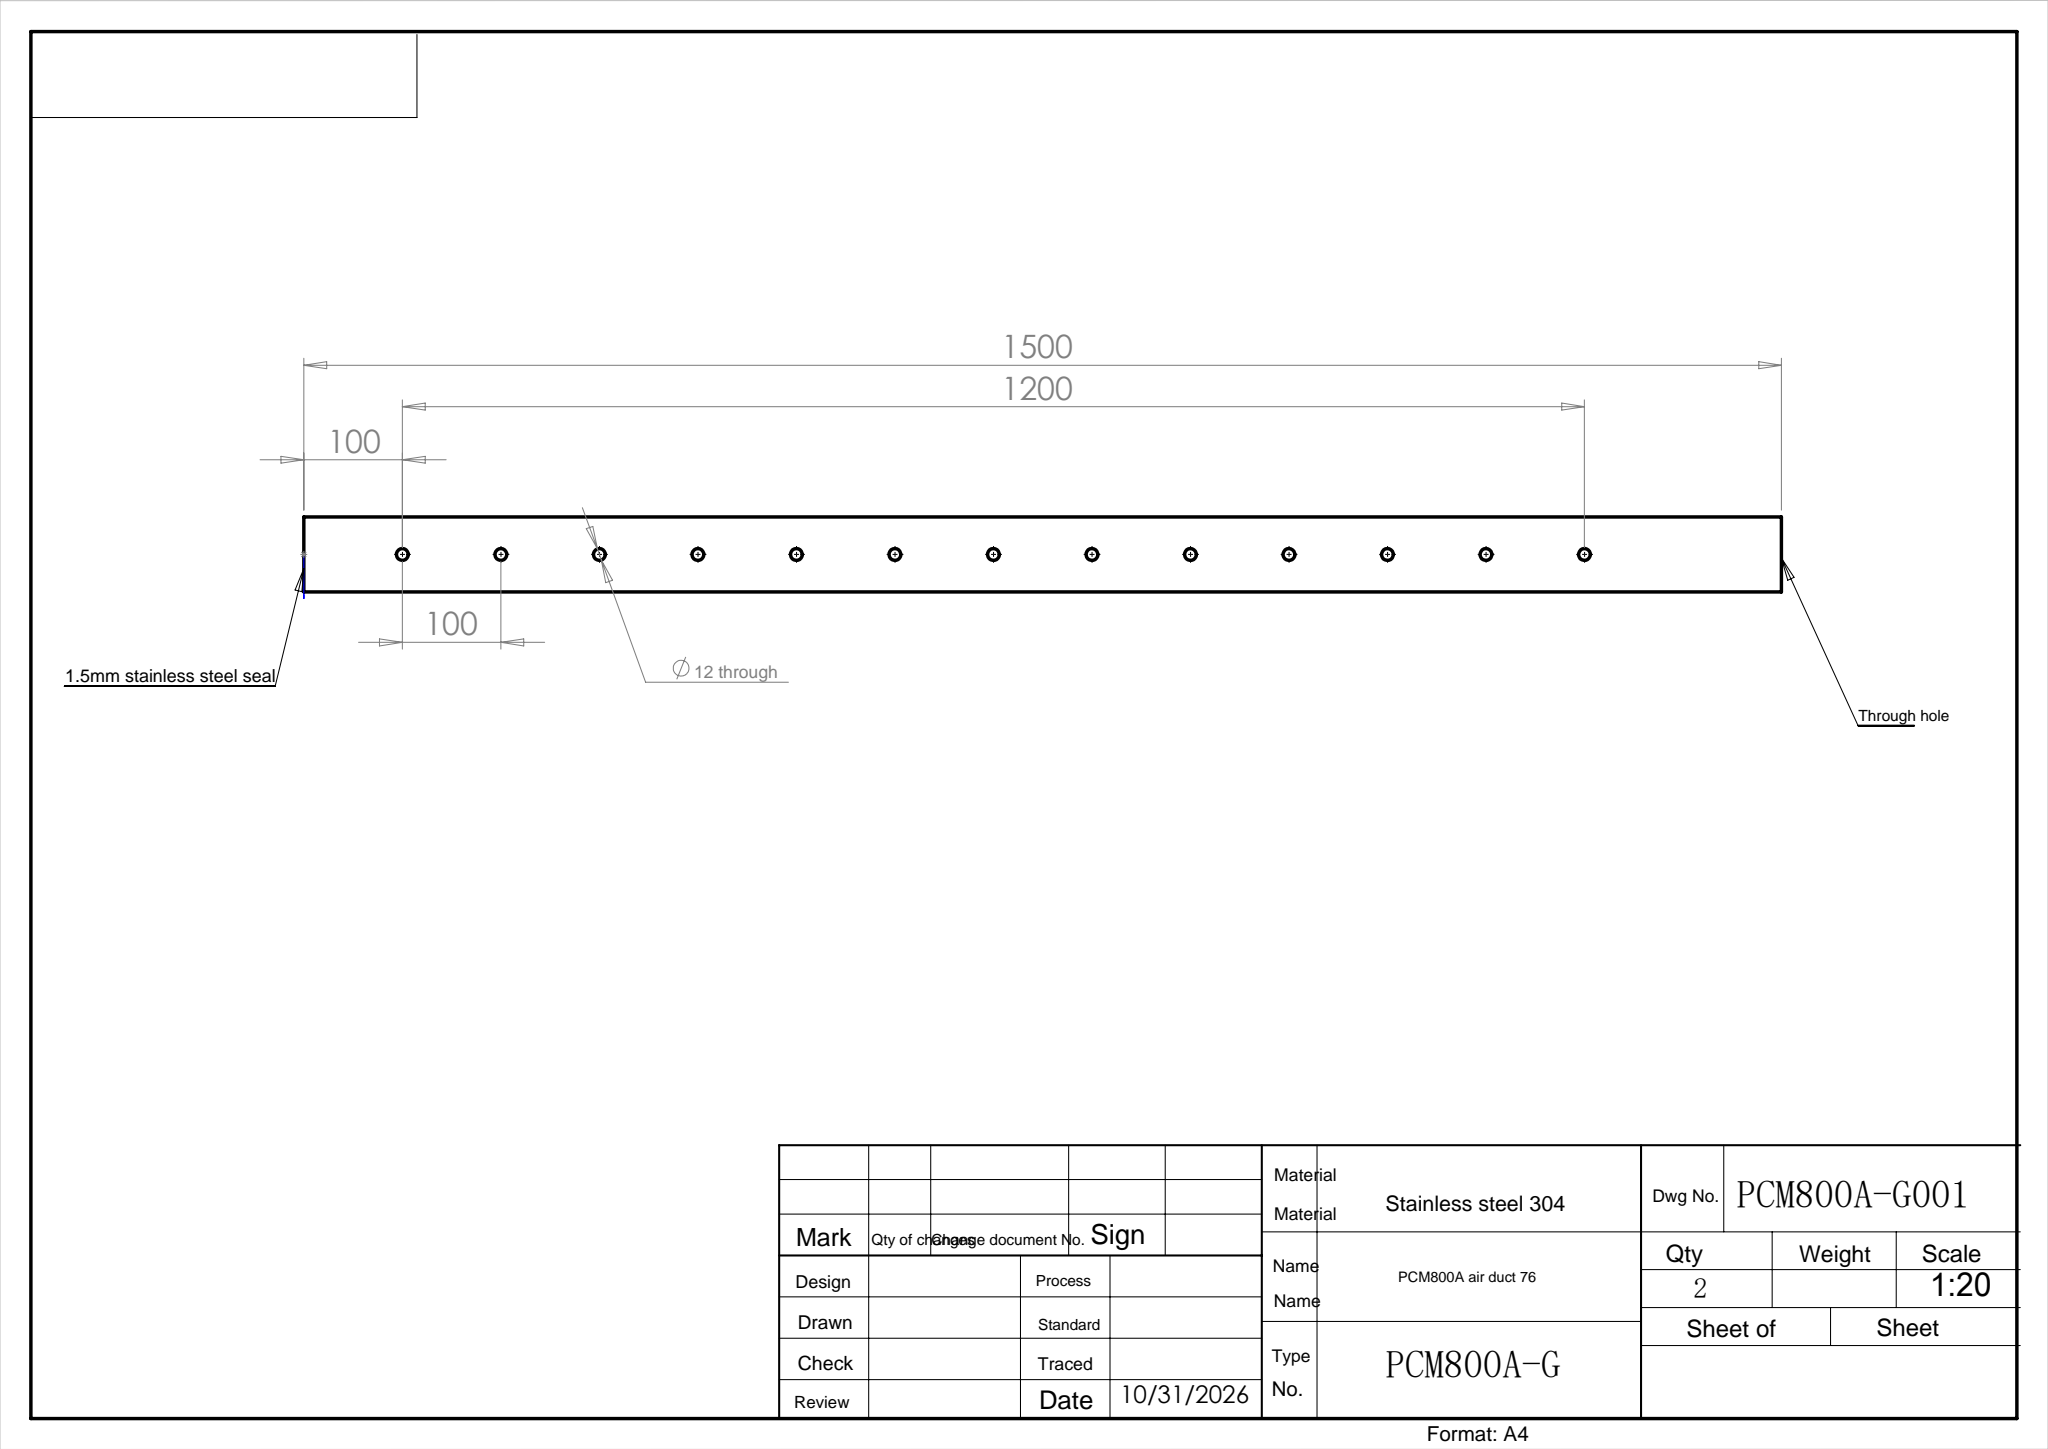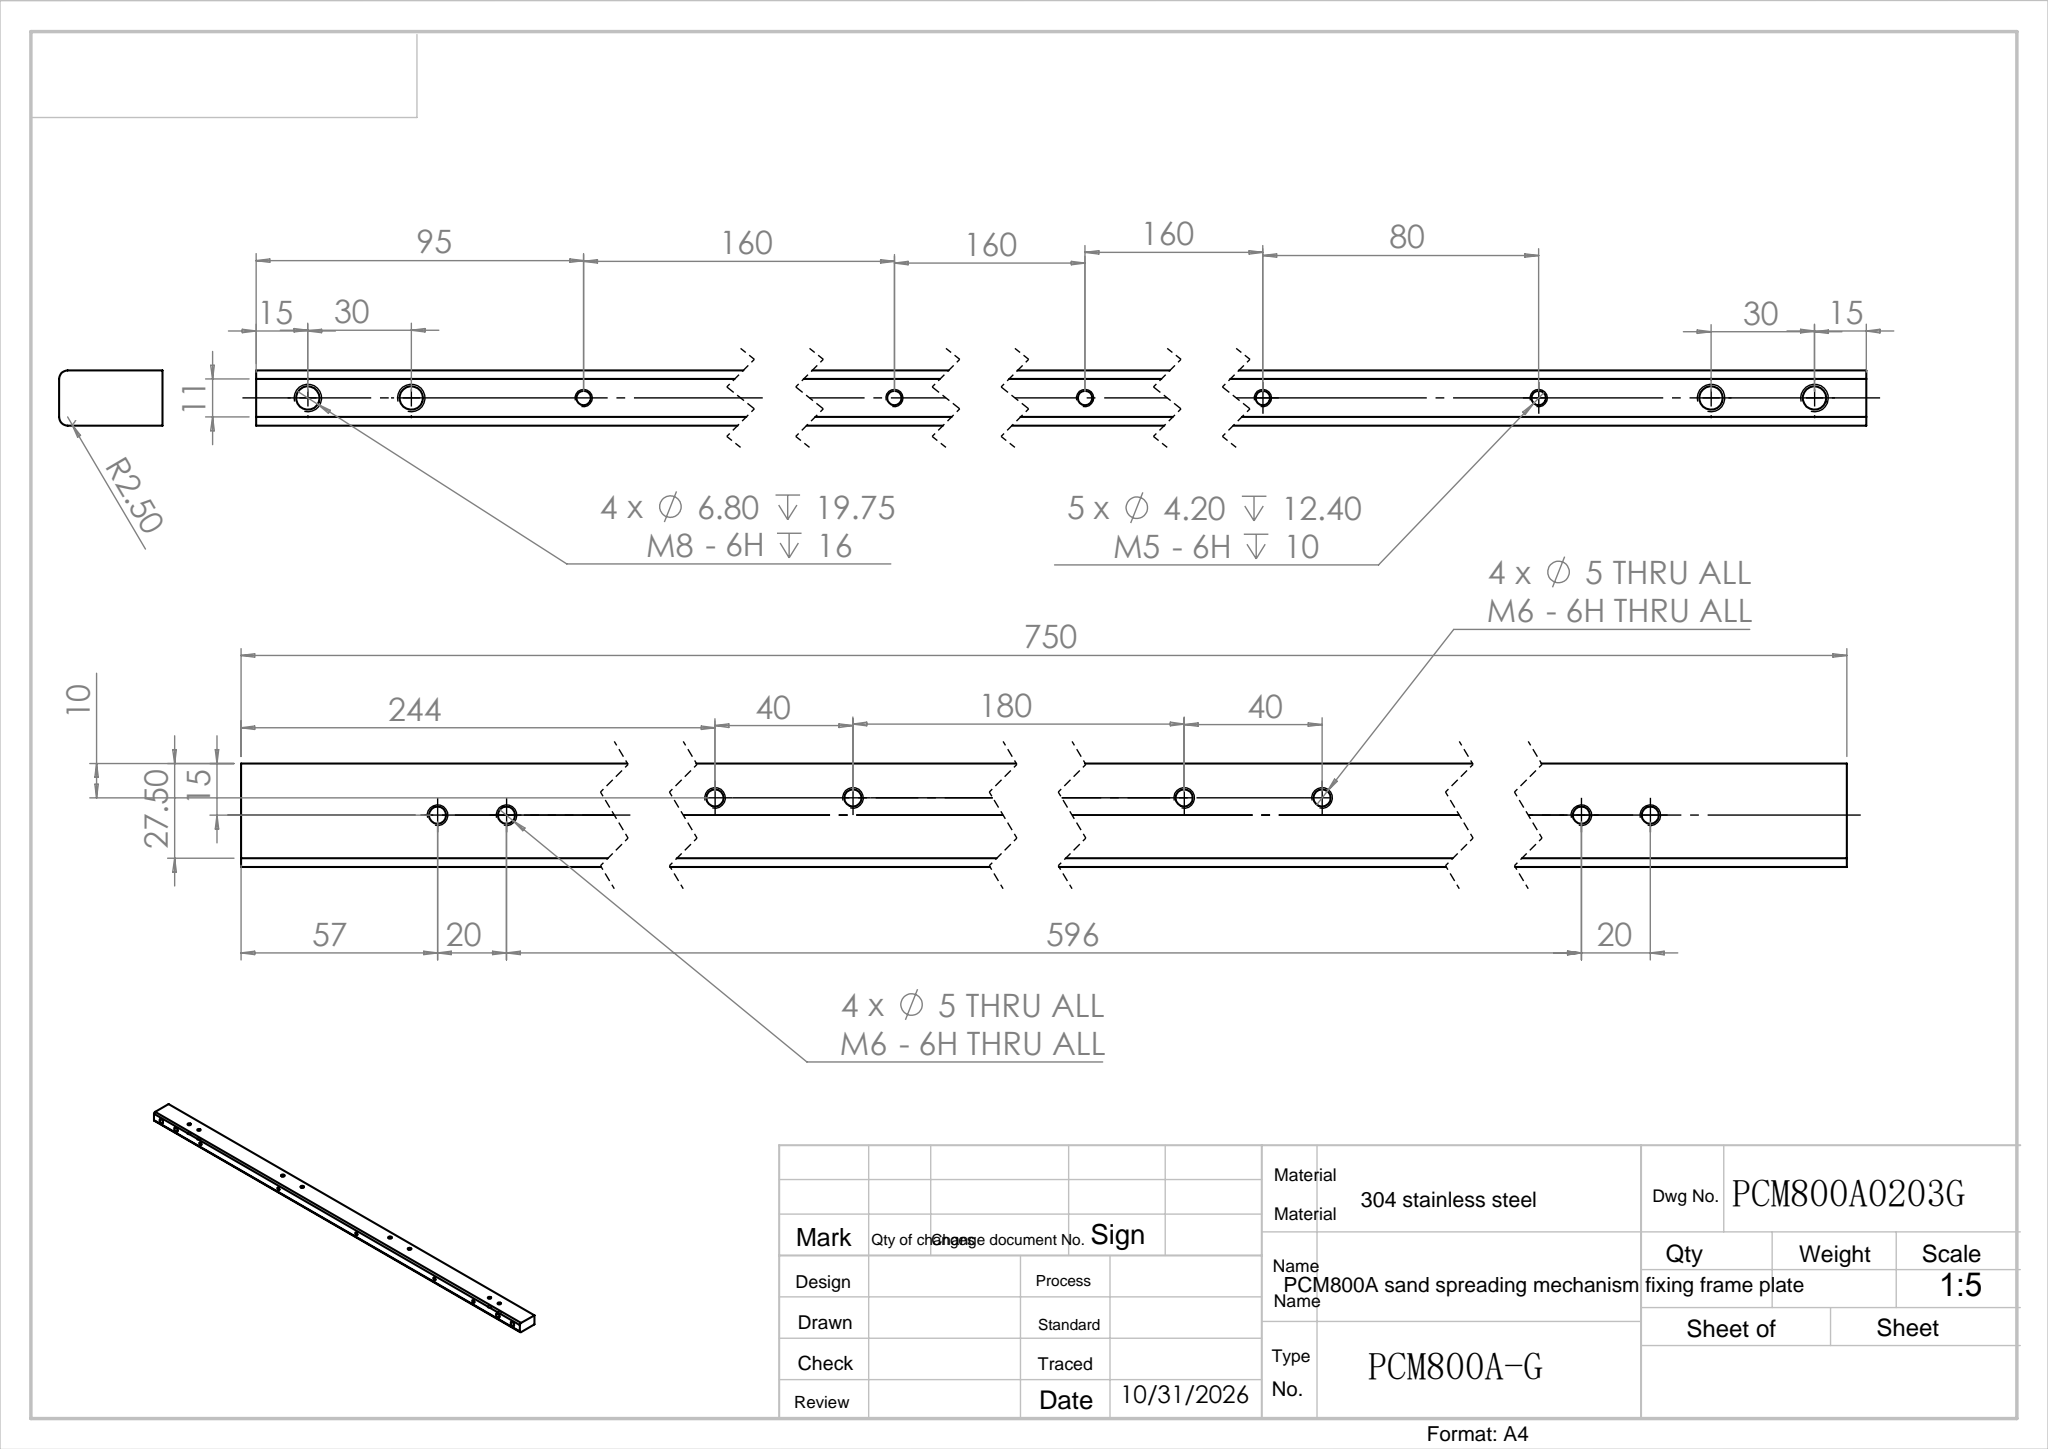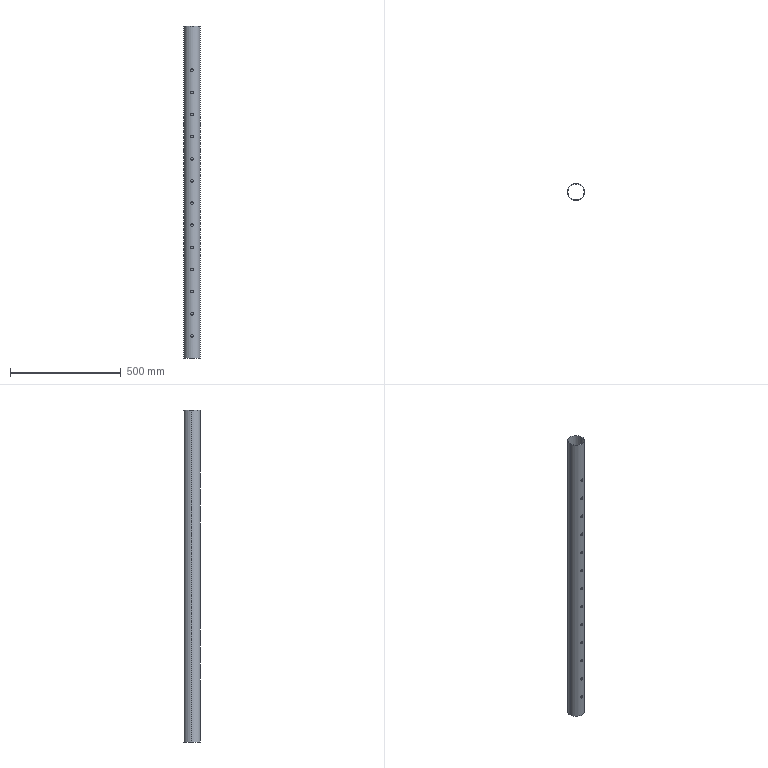Part | SolidWorks | features Extrusion 1, ICE 1 | 1 solid | 32 faces | box 76 x 76 x 1500 mm | volume 351954 mm3 | cylinder 30 | plane 2 | commonest cylinder face diameters 12 x26 74 x2 76 x2